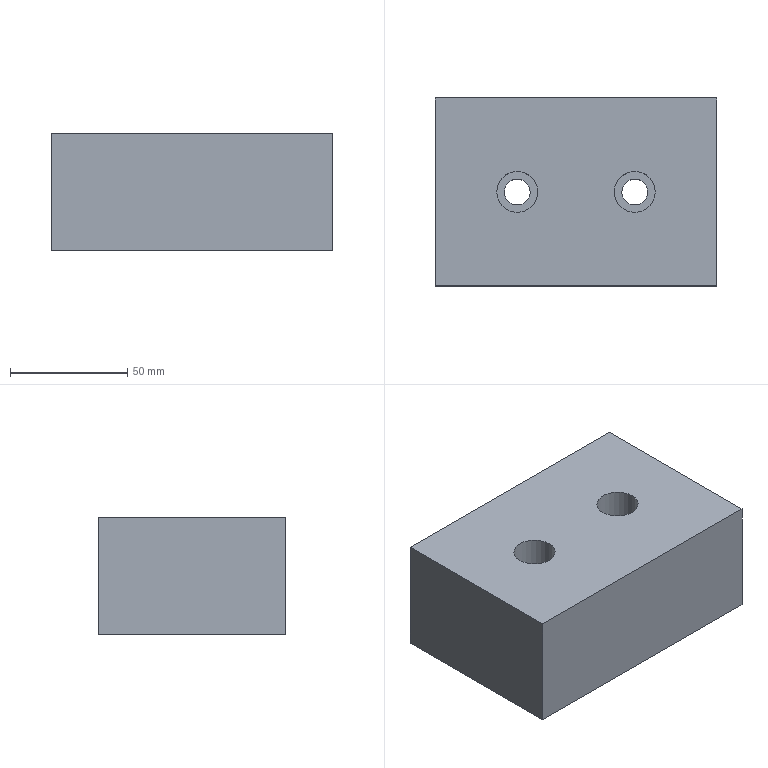Part | NX | features solid 2 | 1 solid | 12 faces | box 120 x 80 x 50 mm | volume 458857 mm3 | plane 8 | cylinder 4 | commonest cylinder face diameters 11 x2 17.5 x2
STEP:
#1=CARTESIAN_POINT('',(1030.,-405.,-30.));
#2=VERTEX_POINT('',#1);
#3=CARTESIAN_POINT('',(1030.,-325.,-30.));
#4=VERTEX_POINT('',#3);
#5=CARTESIAN_POINT('',(1030.,-395.,-30.));
#6=DIRECTION('',(0.,1.,0.));
#7=VECTOR('',#6,1000.);
#8=LINE('',#5,#7);
#9=EDGE_CURVE('',#2,#4,#8,.T.);
#10=ORIENTED_EDGE('',*,*,#9,.T.);
#11=CARTESIAN_POINT('',(1030.,-325.,20.));
#12=VERTEX_POINT('',#11);
#13=CARTESIAN_POINT('',(1030.,-325.,50.));
#14=DIRECTION('',(0.,0.,-1.));
#15=VECTOR('',#14,1000.);
#16=LINE('',#13,#15);
#17=EDGE_CURVE('',#12,#4,#16,.T.);
#18=ORIENTED_EDGE('',*,*,#17,.F.);
#19=CARTESIAN_POINT('',(1030.,-405.,20.));
#20=VERTEX_POINT('',#19);
#21=CARTESIAN_POINT('',(1030.,-395.,20.));
#22=DIRECTION('',(0.,1.,0.));
#23=VECTOR('',#22,1000.);
#24=LINE('',#21,#23);
#25=EDGE_CURVE('',#20,#12,#24,.T.);
#26=ORIENTED_EDGE('',*,*,#25,.F.);
#27=CARTESIAN_POINT('',(1030.,-405.,50.));
#28=DIRECTION('',(0.,0.,-1.));
#29=VECTOR('',#28,1000.);
#30=LINE('',#27,#29);
#31=EDGE_CURVE('',#20,#2,#30,.T.);
#32=ORIENTED_EDGE('',*,*,#31,.T.);
#33=EDGE_LOOP('',(#10,#18,#26,#32));
#34=FACE_BOUND('',#33,.T.);
#35=CARTESIAN_POINT('',(1030.,-395.,50.));
#36=DIRECTION('',(1.,0.,0.));
#37=DIRECTION('',(0.,-1.,0.));
#38=AXIS2_PLACEMENT_3D('',#35,#36,#37);
#39=PLANE('',#38);
#40=ADVANCED_FACE('',(#34),#39,.T.);
#41=CARTESIAN_POINT('',(910.,-325.,-30.));
#42=VERTEX_POINT('',#41);
#43=CARTESIAN_POINT('',(1037.,-325.,-30.));
#44=DIRECTION('',(-1.,0.,0.));
#45=VECTOR('',#44,1000.);
#46=LINE('',#43,#45);
#47=EDGE_CURVE('',#4,#42,#46,.T.);
#48=ORIENTED_EDGE('',*,*,#47,.T.);
#49=CARTESIAN_POINT('',(910.,-325.,20.));
#50=VERTEX_POINT('',#49);
#51=CARTESIAN_POINT('',(910.,-325.,50.));
#52=DIRECTION('',(0.,0.,-1.));
#53=VECTOR('',#52,1000.);
#54=LINE('',#51,#53);
#55=EDGE_CURVE('',#50,#42,#54,.T.);
#56=ORIENTED_EDGE('',*,*,#55,.F.);
#57=CARTESIAN_POINT('',(1037.,-325.,20.));
#58=DIRECTION('',(-1.,0.,0.));
#59=VECTOR('',#58,1000.);
#60=LINE('',#57,#59);
#61=EDGE_CURVE('',#12,#50,#60,.T.);
#62=ORIENTED_EDGE('',*,*,#61,.F.);
#63=ORIENTED_EDGE('',*,*,#17,.T.);
#64=EDGE_LOOP('',(#48,#56,#62,#63));
#65=FACE_BOUND('',#64,.T.);
#66=CARTESIAN_POINT('',(1037.,-325.,50.));
#67=DIRECTION('',(0.,1.,0.));
#68=DIRECTION('',(0.,0.,1.));
#69=AXIS2_PLACEMENT_3D('',#66,#67,#68);
#70=PLANE('',#69);
#71=ADVANCED_FACE('',(#65),#70,.T.);
#72=CARTESIAN_POINT('',(910.,-405.,-30.));
#73=VERTEX_POINT('',#72);
#74=CARTESIAN_POINT('',(910.,-395.,-30.));
#75=DIRECTION('',(0.,-1.,0.));
#76=VECTOR('',#75,1000.);
#77=LINE('',#74,#76);
#78=EDGE_CURVE('',#42,#73,#77,.T.);
#79=ORIENTED_EDGE('',*,*,#78,.T.);
#80=CARTESIAN_POINT('',(910.,-405.,20.));
#81=VERTEX_POINT('',#80);
#82=CARTESIAN_POINT('',(910.,-405.,50.));
#83=DIRECTION('',(0.,0.,-1.));
#84=VECTOR('',#83,1000.);
#85=LINE('',#82,#84);
#86=EDGE_CURVE('',#81,#73,#85,.T.);
#87=ORIENTED_EDGE('',*,*,#86,.F.);
#88=CARTESIAN_POINT('',(910.,-325.,20.));
#89=DIRECTION('',(0.,-1.,0.));
#90=VECTOR('',#89,1000.);
#91=LINE('',#88,#90);
#92=EDGE_CURVE('',#50,#81,#91,.T.);
#93=ORIENTED_EDGE('',*,*,#92,.F.);
#94=ORIENTED_EDGE('',*,*,#55,.T.);
#95=EDGE_LOOP('',(#79,#87,#93,#94));
#96=FACE_BOUND('',#95,.T.);
#97=CARTESIAN_POINT('',(910.,-325.,50.));
#98=DIRECTION('',(-1.,0.,0.));
#99=DIRECTION('',(0.,1.,0.));
#100=AXIS2_PLACEMENT_3D('',#97,#98,#99);
#101=PLANE('',#100);
#102=ADVANCED_FACE('',(#96),#101,.T.);
#103=CARTESIAN_POINT('',(1037.,-405.,-30.));
#104=DIRECTION('',(1.,0.,0.));
#105=VECTOR('',#104,1000.);
#106=LINE('',#103,#105);
#107=EDGE_CURVE('',#73,#2,#106,.T.);
#108=ORIENTED_EDGE('',*,*,#107,.T.);
#109=ORIENTED_EDGE('',*,*,#31,.F.);
#110=CARTESIAN_POINT('',(910.,-405.,20.));
#111=DIRECTION('',(1.,0.,0.));
#112=VECTOR('',#111,1000.);
#113=LINE('',#110,#112);
#114=EDGE_CURVE('',#81,#20,#113,.T.);
#115=ORIENTED_EDGE('',*,*,#114,.F.);
#116=ORIENTED_EDGE('',*,*,#86,.T.);
#117=EDGE_LOOP('',(#108,#109,#115,#116));
#118=FACE_BOUND('',#117,.T.);
#119=CARTESIAN_POINT('',(910.,-405.,50.));
#120=DIRECTION('',(0.,-1.,0.));
#121=DIRECTION('',(-1.,0.,0.));
#122=AXIS2_PLACEMENT_3D('',#119,#120,#121);
#123=PLANE('',#122);
#124=ADVANCED_FACE('',(#118),#123,.T.);
#125=CARTESIAN_POINT('',(986.25,-365.,20.));
#126=VERTEX_POINT('',#125);
#127=CARTESIAN_POINT('',(995.,-365.,20.));
#128=DIRECTION('',(0.,0.,-1.));
#129=DIRECTION('',(-1.,0.,0.));
#130=AXIS2_PLACEMENT_3D('',#127,#128,#129);
#131=CIRCLE('',#130,8.75);
#132=EDGE_CURVE('',#126,#126,#131,.T.);
#133=ORIENTED_EDGE('',*,*,#132,.T.);
#134=EDGE_LOOP('',(#133));
#135=FACE_BOUND('',#134,.T.);
#136=CARTESIAN_POINT('',(936.25,-365.,20.));
#137=VERTEX_POINT('',#136);
#138=CARTESIAN_POINT('',(945.,-365.,20.));
#139=DIRECTION('',(0.,0.,-1.));
#140=DIRECTION('',(-1.,0.,0.));
#141=AXIS2_PLACEMENT_3D('',#138,#139,#140);
#142=CIRCLE('',#141,8.75);
#143=EDGE_CURVE('',#137,#137,#142,.F.);
#144=ORIENTED_EDGE('',*,*,#143,.F.);
#145=EDGE_LOOP('',(#144));
#146=FACE_BOUND('',#145,.T.);
#147=ORIENTED_EDGE('',*,*,#25,.T.);
#148=ORIENTED_EDGE('',*,*,#61,.T.);
#149=ORIENTED_EDGE('',*,*,#92,.T.);
#150=ORIENTED_EDGE('',*,*,#114,.T.);
#151=EDGE_LOOP('',(#147,#148,#149,#150));
#152=FACE_BOUND('',#151,.T.);
#153=CARTESIAN_POINT('',(1037.,-395.,20.));
#154=DIRECTION('',(0.,0.,1.));
#155=DIRECTION('',(-1.,0.,0.));
#156=AXIS2_PLACEMENT_3D('',#153,#154,#155);
#157=PLANE('',#156);
#158=ADVANCED_FACE('',(#135,#146,#152),#157,.T.);
#159=CARTESIAN_POINT('',(989.5,-365.,-30.));
#160=VERTEX_POINT('',#159);
#161=CARTESIAN_POINT('',(995.,-365.,-30.));
#162=DIRECTION('',(0.,0.,1.));
#163=DIRECTION('',(-1.,0.,0.));
#164=AXIS2_PLACEMENT_3D('',#161,#162,#163);
#165=CIRCLE('',#164,5.5);
#166=EDGE_CURVE('',#160,#160,#165,.F.);
#167=ORIENTED_EDGE('',*,*,#166,.F.);
#168=EDGE_LOOP('',(#167));
#169=FACE_BOUND('',#168,.T.);
#170=CARTESIAN_POINT('',(939.5,-365.,-30.));
#171=VERTEX_POINT('',#170);
#172=CARTESIAN_POINT('',(945.,-365.,-30.));
#173=DIRECTION('',(0.,0.,1.));
#174=DIRECTION('',(-1.,0.,0.));
#175=AXIS2_PLACEMENT_3D('',#172,#173,#174);
#176=CIRCLE('',#175,5.5);
#177=EDGE_CURVE('',#171,#171,#176,.F.);
#178=ORIENTED_EDGE('',*,*,#177,.F.);
#179=EDGE_LOOP('',(#178));
#180=FACE_BOUND('',#179,.T.);
#181=ORIENTED_EDGE('',*,*,#9,.F.);
#182=ORIENTED_EDGE('',*,*,#107,.F.);
#183=ORIENTED_EDGE('',*,*,#78,.F.);
#184=ORIENTED_EDGE('',*,*,#47,.F.);
#185=EDGE_LOOP('',(#181,#182,#183,#184));
#186=FACE_BOUND('',#185,.T.);
#187=CARTESIAN_POINT('',(1037.,-395.,-30.));
#188=DIRECTION('',(0.,0.,1.));
#189=DIRECTION('',(-1.,0.,0.));
#190=AXIS2_PLACEMENT_3D('',#187,#188,#189);
#191=PLANE('',#190);
#192=ADVANCED_FACE('',(#169,#180,#186),#191,.F.);
#193=CARTESIAN_POINT('',(950.5,-365.,-20.));
#194=VERTEX_POINT('',#193);
#195=CARTESIAN_POINT('',(945.,-365.,-20.));
#196=DIRECTION('',(0.,0.,1.));
#197=DIRECTION('',(1.,0.,0.));
#198=AXIS2_PLACEMENT_3D('',#195,#196,#197);
#199=CIRCLE('',#198,5.5);
#200=EDGE_CURVE('',#194,#194,#199,.T.);
#201=ORIENTED_EDGE('',*,*,#200,.T.);
#202=EDGE_LOOP('',(#201));
#203=FACE_BOUND('',#202,.T.);
#204=ORIENTED_EDGE('',*,*,#177,.T.);
#205=EDGE_LOOP('',(#204));
#206=FACE_BOUND('',#205,.T.);
#207=CARTESIAN_POINT('',(945.,-365.,-80.));
#208=DIRECTION('',(0.,0.,-1.));
#209=DIRECTION('',(1.,0.,0.));
#210=AXIS2_PLACEMENT_3D('',#207,#208,#209);
#211=CYLINDRICAL_SURFACE('',#210,5.5);
#212=ADVANCED_FACE('',(#203,#206),#211,.F.);
#213=ORIENTED_EDGE('',*,*,#200,.F.);
#214=EDGE_LOOP('',(#213));
#215=FACE_BOUND('',#214,.T.);
#216=CARTESIAN_POINT('',(953.75,-365.,-20.));
#217=VERTEX_POINT('',#216);
#218=CARTESIAN_POINT('',(945.,-365.,-20.));
#219=DIRECTION('',(0.,0.,1.));
#220=DIRECTION('',(1.,0.,0.));
#221=AXIS2_PLACEMENT_3D('',#218,#219,#220);
#222=CIRCLE('',#221,8.75);
#223=EDGE_CURVE('',#217,#217,#222,.T.);
#224=ORIENTED_EDGE('',*,*,#223,.T.);
#225=EDGE_LOOP('',(#224));
#226=FACE_BOUND('',#225,.T.);
#227=CARTESIAN_POINT('',(945.,-360.,-20.));
#228=DIRECTION('',(0.,0.,-1.));
#229=DIRECTION('',(1.,0.,0.));
#230=AXIS2_PLACEMENT_3D('',#227,#228,#229);
#231=PLANE('',#230);
#232=ADVANCED_FACE('',(#215,#226),#231,.F.);
#233=ORIENTED_EDGE('',*,*,#223,.F.);
#234=EDGE_LOOP('',(#233));
#235=FACE_BOUND('',#234,.T.);
#236=ORIENTED_EDGE('',*,*,#143,.T.);
#237=EDGE_LOOP('',(#236));
#238=FACE_BOUND('',#237,.T.);
#239=CARTESIAN_POINT('',(945.,-365.,50.));
#240=DIRECTION('',(0.,0.,-1.));
#241=DIRECTION('',(1.,0.,0.));
#242=AXIS2_PLACEMENT_3D('',#239,#240,#241);
#243=CYLINDRICAL_SURFACE('',#242,8.75);
#244=ADVANCED_FACE('',(#235,#238),#243,.F.);
#245=CARTESIAN_POINT('',(989.5,-365.,-20.));
#246=VERTEX_POINT('',#245);
#247=CARTESIAN_POINT('',(995.,-365.,-20.));
#248=DIRECTION('',(0.,0.,-1.));
#249=DIRECTION('',(-1.,0.,0.));
#250=AXIS2_PLACEMENT_3D('',#247,#248,#249);
#251=CIRCLE('',#250,5.5);
#252=EDGE_CURVE('',#246,#246,#251,.T.);
#253=ORIENTED_EDGE('',*,*,#252,.F.);
#254=EDGE_LOOP('',(#253));
#255=FACE_BOUND('',#254,.T.);
#256=ORIENTED_EDGE('',*,*,#166,.T.);
#257=EDGE_LOOP('',(#256));
#258=FACE_BOUND('',#257,.T.);
#259=CARTESIAN_POINT('',(995.,-365.,-80.));
#260=DIRECTION('',(0.,0.,-1.));
#261=DIRECTION('',(-1.,0.,0.));
#262=AXIS2_PLACEMENT_3D('',#259,#260,#261);
#263=CYLINDRICAL_SURFACE('',#262,5.5);
#264=ADVANCED_FACE('',(#255,#258),#263,.F.);
#265=ORIENTED_EDGE('',*,*,#252,.T.);
#266=EDGE_LOOP('',(#265));
#267=FACE_BOUND('',#266,.T.);
#268=CARTESIAN_POINT('',(986.25,-365.,-20.));
#269=VERTEX_POINT('',#268);
#270=CARTESIAN_POINT('',(995.,-365.,-20.));
#271=DIRECTION('',(0.,0.,-1.));
#272=DIRECTION('',(-1.,0.,0.));
#273=AXIS2_PLACEMENT_3D('',#270,#271,#272);
#274=CIRCLE('',#273,8.75);
#275=EDGE_CURVE('',#269,#269,#274,.T.);
#276=ORIENTED_EDGE('',*,*,#275,.F.);
#277=EDGE_LOOP('',(#276));
#278=FACE_BOUND('',#277,.T.);
#279=CARTESIAN_POINT('',(1002.,-360.,-20.));
#280=DIRECTION('',(0.,0.,-1.));
#281=DIRECTION('',(-1.,0.,0.));
#282=AXIS2_PLACEMENT_3D('',#279,#280,#281);
#283=PLANE('',#282);
#284=ADVANCED_FACE('',(#267,#278),#283,.F.);
#285=ORIENTED_EDGE('',*,*,#275,.T.);
#286=EDGE_LOOP('',(#285));
#287=FACE_BOUND('',#286,.T.);
#288=ORIENTED_EDGE('',*,*,#132,.F.);
#289=EDGE_LOOP('',(#288));
#290=FACE_BOUND('',#289,.T.);
#291=CARTESIAN_POINT('',(995.,-365.,50.));
#292=DIRECTION('',(0.,0.,-1.));
#293=DIRECTION('',(-1.,0.,0.));
#294=AXIS2_PLACEMENT_3D('',#291,#292,#293);
#295=CYLINDRICAL_SURFACE('',#294,8.75);
#296=ADVANCED_FACE('',(#287,#290),#295,.F.);
#297=CLOSED_SHELL('',(#40,#71,#102,#124,#158,#192,#212,#232,#244,#264,#284,#296));
#298=MANIFOLD_SOLID_BREP('',#297);
#299=(LENGTH_UNIT()NAMED_UNIT(*)SI_UNIT(.MILLI.,.METRE.));
#300=UNCERTAINTY_MEASURE_WITH_UNIT(LENGTH_MEASURE(0.00001),#299,'','');
#301=(NAMED_UNIT(*)PLANE_ANGLE_UNIT()SI_UNIT($,.RADIAN.));
#302=(NAMED_UNIT(*)SI_UNIT($,.STERADIAN.)SOLID_ANGLE_UNIT());
#303=(GEOMETRIC_REPRESENTATION_CONTEXT(3)GLOBAL_UNCERTAINTY_ASSIGNED_CONTEXT((#300))GLOBAL_UNIT_ASSIGNED_CONTEXT((#299,#301,#302))REPRESENTATION_CONTEXT('',''));
#304=ADVANCED_BREP_SHAPE_REPRESENTATION('',(#298),#303);